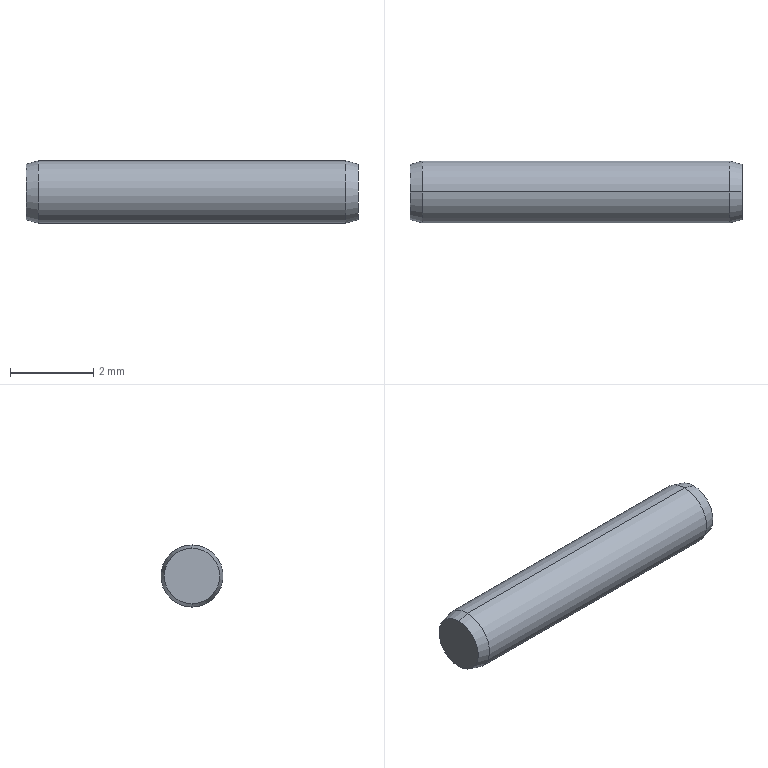Part | STEP file | parallel pins unhardening steel gb_GB_CONNECTING_PIECE_PIN_PPUS 1.5X8.step.STEP.STEP.STEP.STEP-562.STEP | 1 solid | 8 faces | box 8 x 1.5 x 1.5 mm | volume 14.028 mm3 | cone 4 | cylinder 2 | plane 2 | commonest cylinder face diameters 1.5 x2
STEP:
#1=CARTESIAN_POINT('',(0.,0.,0.6696));
#2=VERTEX_POINT('',#1);
#3=CARTESIAN_POINT('',(0.,0.,-0.6696));
#4=VERTEX_POINT('',#3);
#5=CARTESIAN_POINT('',(0.,0.,0.));
#6=DIRECTION('',(-1.,0.,0.));
#7=DIRECTION('',(0.,0.,1.));
#8=AXIS2_PLACEMENT_3D('',#5,#6,#7);
#9=CIRCLE('',#8,0.6696);
#10=EDGE_CURVE('',#2,#4,#9,.T.);
#11=ORIENTED_EDGE('',*,*,#10,.F.);
#12=CARTESIAN_POINT('',(0.3,0.,0.75));
#13=VERTEX_POINT('',#12);
#14=CARTESIAN_POINT('',(0.3,0.,0.75));
#15=DIRECTION('',(0.9659,0.,0.2588));
#16=VECTOR('',#15,1000.);
#17=LINE('',#14,#16);
#18=EDGE_CURVE('',#2,#13,#17,.T.);
#19=ORIENTED_EDGE('',*,*,#18,.T.);
#20=CARTESIAN_POINT('',(0.3,0.,-0.75));
#21=VERTEX_POINT('',#20);
#22=CARTESIAN_POINT('',(0.3,0.,0.));
#23=DIRECTION('',(-1.,0.,0.));
#24=DIRECTION('',(0.,0.,1.));
#25=AXIS2_PLACEMENT_3D('',#22,#23,#24);
#26=CIRCLE('',#25,0.75);
#27=EDGE_CURVE('',#13,#21,#26,.T.);
#28=ORIENTED_EDGE('',*,*,#27,.T.);
#29=CARTESIAN_POINT('',(0.3,0.,-0.75));
#30=DIRECTION('',(0.9659,0.,-0.2588));
#31=VECTOR('',#30,1000.);
#32=LINE('',#29,#31);
#33=EDGE_CURVE('',#4,#21,#32,.T.);
#34=ORIENTED_EDGE('',*,*,#33,.F.);
#35=EDGE_LOOP('',(#11,#19,#28,#34));
#36=FACE_OUTER_BOUND('',#35,.T.);
#37=CARTESIAN_POINT('',(0.3,0.,0.));
#38=DIRECTION('',(1.,0.,0.));
#39=DIRECTION('',(0.,0.,-1.));
#40=AXIS2_PLACEMENT_3D('',#37,#38,#39);
#41=CONICAL_SURFACE('',#40,0.75,0.2618);
#42=ADVANCED_FACE('',(#36),#41,.T.);
#43=CARTESIAN_POINT('',(7.7,0.,0.75));
#44=VERTEX_POINT('',#43);
#45=CARTESIAN_POINT('',(7.7,0.,-0.75));
#46=VERTEX_POINT('',#45);
#47=CARTESIAN_POINT('',(7.7,0.,0.));
#48=DIRECTION('',(-1.,0.,0.));
#49=DIRECTION('',(0.,0.,1.));
#50=AXIS2_PLACEMENT_3D('',#47,#48,#49);
#51=CIRCLE('',#50,0.75);
#52=EDGE_CURVE('',#44,#46,#51,.T.);
#53=ORIENTED_EDGE('',*,*,#52,.T.);
#54=CARTESIAN_POINT('',(-1.656,0.,-0.75));
#55=DIRECTION('',(-1.,0.,0.));
#56=VECTOR('',#55,1000.);
#57=LINE('',#54,#56);
#58=EDGE_CURVE('',#46,#21,#57,.T.);
#59=ORIENTED_EDGE('',*,*,#58,.T.);
#60=ORIENTED_EDGE('',*,*,#27,.F.);
#61=CARTESIAN_POINT('',(-1.656,0.,0.75));
#62=DIRECTION('',(-1.,0.,0.));
#63=VECTOR('',#62,1000.);
#64=LINE('',#61,#63);
#65=EDGE_CURVE('',#44,#13,#64,.T.);
#66=ORIENTED_EDGE('',*,*,#65,.F.);
#67=EDGE_LOOP('',(#53,#59,#60,#66));
#68=FACE_OUTER_BOUND('',#67,.T.);
#69=CARTESIAN_POINT('',(-1.656,0.,0.));
#70=DIRECTION('',(-1.,0.,0.));
#71=DIRECTION('',(0.,0.,1.));
#72=AXIS2_PLACEMENT_3D('',#69,#70,#71);
#73=CYLINDRICAL_SURFACE('',#72,0.75);
#74=ADVANCED_FACE('',(#68),#73,.T.);
#75=CARTESIAN_POINT('',(8.,0.,0.6696));
#76=VERTEX_POINT('',#75);
#77=CARTESIAN_POINT('',(8.,0.,-0.6696));
#78=VERTEX_POINT('',#77);
#79=CARTESIAN_POINT('',(8.,0.,0.));
#80=DIRECTION('',(-1.,0.,0.));
#81=DIRECTION('',(0.,0.,1.));
#82=AXIS2_PLACEMENT_3D('',#79,#80,#81);
#83=CIRCLE('',#82,0.6696);
#84=EDGE_CURVE('',#76,#78,#83,.T.);
#85=ORIENTED_EDGE('',*,*,#84,.T.);
#86=CARTESIAN_POINT('',(8.,0.,-0.6696));
#87=DIRECTION('',(-0.9659,0.,-0.2588));
#88=VECTOR('',#87,1000.);
#89=LINE('',#86,#88);
#90=EDGE_CURVE('',#78,#46,#89,.T.);
#91=ORIENTED_EDGE('',*,*,#90,.T.);
#92=ORIENTED_EDGE('',*,*,#52,.F.);
#93=CARTESIAN_POINT('',(8.,0.,0.6696));
#94=DIRECTION('',(-0.9659,0.,0.2588));
#95=VECTOR('',#94,1000.);
#96=LINE('',#93,#95);
#97=EDGE_CURVE('',#76,#44,#96,.T.);
#98=ORIENTED_EDGE('',*,*,#97,.F.);
#99=EDGE_LOOP('',(#85,#91,#92,#98));
#100=FACE_OUTER_BOUND('',#99,.T.);
#101=CARTESIAN_POINT('',(8.,0.,0.));
#102=DIRECTION('',(-1.,0.,0.));
#103=DIRECTION('',(0.,0.,1.));
#104=AXIS2_PLACEMENT_3D('',#101,#102,#103);
#105=CONICAL_SURFACE('',#104,0.6696,0.2618);
#106=ADVANCED_FACE('',(#100),#105,.T.);
#107=CARTESIAN_POINT('',(0.,0.,0.));
#108=DIRECTION('',(-1.,0.,0.));
#109=DIRECTION('',(0.,0.,1.));
#110=AXIS2_PLACEMENT_3D('',#107,#108,#109);
#111=CIRCLE('',#110,0.6696);
#112=EDGE_CURVE('',#4,#2,#111,.T.);
#113=ORIENTED_EDGE('',*,*,#112,.T.);
#114=ORIENTED_EDGE('',*,*,#10,.T.);
#115=EDGE_LOOP('',(#113,#114));
#116=FACE_OUTER_BOUND('',#115,.T.);
#117=CARTESIAN_POINT('',(0.,0.6696,0.));
#118=DIRECTION('',(1.,0.,0.));
#119=DIRECTION('',(0.,1.,0.));
#120=AXIS2_PLACEMENT_3D('',#117,#118,#119);
#121=PLANE('',#120);
#122=ADVANCED_FACE('',(#116),#121,.F.);
#123=ORIENTED_EDGE('',*,*,#84,.F.);
#124=CARTESIAN_POINT('',(8.,0.,0.));
#125=DIRECTION('',(-1.,0.,0.));
#126=DIRECTION('',(0.,0.,1.));
#127=AXIS2_PLACEMENT_3D('',#124,#125,#126);
#128=CIRCLE('',#127,0.6696);
#129=EDGE_CURVE('',#78,#76,#128,.T.);
#130=ORIENTED_EDGE('',*,*,#129,.F.);
#131=EDGE_LOOP('',(#123,#130));
#132=FACE_OUTER_BOUND('',#131,.T.);
#133=CARTESIAN_POINT('',(8.,0.,0.));
#134=DIRECTION('',(-1.,0.,0.));
#135=DIRECTION('',(0.,0.,1.));
#136=AXIS2_PLACEMENT_3D('',#133,#134,#135);
#137=PLANE('',#136);
#138=ADVANCED_FACE('',(#132),#137,.F.);
#139=ORIENTED_EDGE('',*,*,#90,.F.);
#140=ORIENTED_EDGE('',*,*,#129,.T.);
#141=ORIENTED_EDGE('',*,*,#97,.T.);
#142=CARTESIAN_POINT('',(7.7,0.,0.));
#143=DIRECTION('',(-1.,0.,0.));
#144=DIRECTION('',(0.,0.,1.));
#145=AXIS2_PLACEMENT_3D('',#142,#143,#144);
#146=CIRCLE('',#145,0.75);
#147=EDGE_CURVE('',#46,#44,#146,.T.);
#148=ORIENTED_EDGE('',*,*,#147,.F.);
#149=EDGE_LOOP('',(#139,#140,#141,#148));
#150=FACE_OUTER_BOUND('',#149,.T.);
#151=CARTESIAN_POINT('',(8.,0.,0.));
#152=DIRECTION('',(-1.,0.,0.));
#153=DIRECTION('',(0.,0.,1.));
#154=AXIS2_PLACEMENT_3D('',#151,#152,#153);
#155=CONICAL_SURFACE('',#154,0.6696,0.2618);
#156=ADVANCED_FACE('',(#150),#155,.T.);
#157=ORIENTED_EDGE('',*,*,#58,.F.);
#158=ORIENTED_EDGE('',*,*,#147,.T.);
#159=ORIENTED_EDGE('',*,*,#65,.T.);
#160=CARTESIAN_POINT('',(0.3,0.,0.));
#161=DIRECTION('',(-1.,0.,0.));
#162=DIRECTION('',(0.,0.,1.));
#163=AXIS2_PLACEMENT_3D('',#160,#161,#162);
#164=CIRCLE('',#163,0.75);
#165=EDGE_CURVE('',#21,#13,#164,.T.);
#166=ORIENTED_EDGE('',*,*,#165,.F.);
#167=EDGE_LOOP('',(#157,#158,#159,#166));
#168=FACE_OUTER_BOUND('',#167,.T.);
#169=CARTESIAN_POINT('',(-1.656,0.,0.));
#170=DIRECTION('',(-1.,0.,0.));
#171=DIRECTION('',(0.,0.,1.));
#172=AXIS2_PLACEMENT_3D('',#169,#170,#171);
#173=CYLINDRICAL_SURFACE('',#172,0.75);
#174=ADVANCED_FACE('',(#168),#173,.T.);
#175=ORIENTED_EDGE('',*,*,#18,.F.);
#176=ORIENTED_EDGE('',*,*,#112,.F.);
#177=ORIENTED_EDGE('',*,*,#33,.T.);
#178=ORIENTED_EDGE('',*,*,#165,.T.);
#179=EDGE_LOOP('',(#175,#176,#177,#178));
#180=FACE_OUTER_BOUND('',#179,.T.);
#181=CARTESIAN_POINT('',(0.3,0.,0.));
#182=DIRECTION('',(1.,0.,0.));
#183=DIRECTION('',(0.,0.,-1.));
#184=AXIS2_PLACEMENT_3D('',#181,#182,#183);
#185=CONICAL_SURFACE('',#184,0.75,0.2618);
#186=ADVANCED_FACE('',(#180),#185,.T.);
#187=CLOSED_SHELL('',(#42,#74,#106,#122,#138,#156,#174,#186));
#188=MANIFOLD_SOLID_BREP('',#187);
#189=CARTESIAN_POINT('',(0.,0.,0.));
#190=DIRECTION('',(0.,0.,1.));
#191=DIRECTION('',(1.,0.,0.));
#192=AXIS2_PLACEMENT_3D('',#189,#190,#191);
#193=(LENGTH_UNIT()NAMED_UNIT(*)SI_UNIT(.MILLI.,.METRE.));
#194=UNCERTAINTY_MEASURE_WITH_UNIT(LENGTH_MEASURE(0.00001),#193,'','');
#195=(NAMED_UNIT(*)PLANE_ANGLE_UNIT()SI_UNIT($,.RADIAN.));
#196=(NAMED_UNIT(*)SI_UNIT($,.STERADIAN.)SOLID_ANGLE_UNIT());
#197=(GEOMETRIC_REPRESENTATION_CONTEXT(3)GLOBAL_UNCERTAINTY_ASSIGNED_CONTEXT((#194))GLOBAL_UNIT_ASSIGNED_CONTEXT((#193,#195,#196))REPRESENTATION_CONTEXT('',''));
#198=ADVANCED_BREP_SHAPE_REPRESENTATION('',(#188,#192),#197);